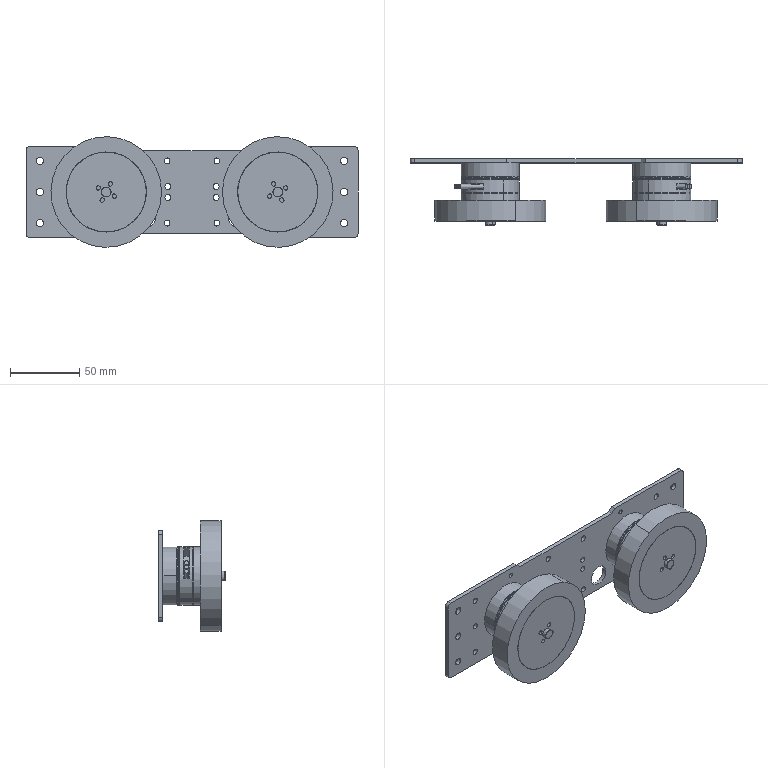Part | SolidWorks | 12 solids | 468 faces | box 240 x 48 x 80 mm | volume 254728 mm3 | cylinder 272 | plane 180 | cone 16 | commonest cylinder face diameters 3 x84 4.2 x56 5.2 x24 3.1 x16 3.2 x16 42 x16